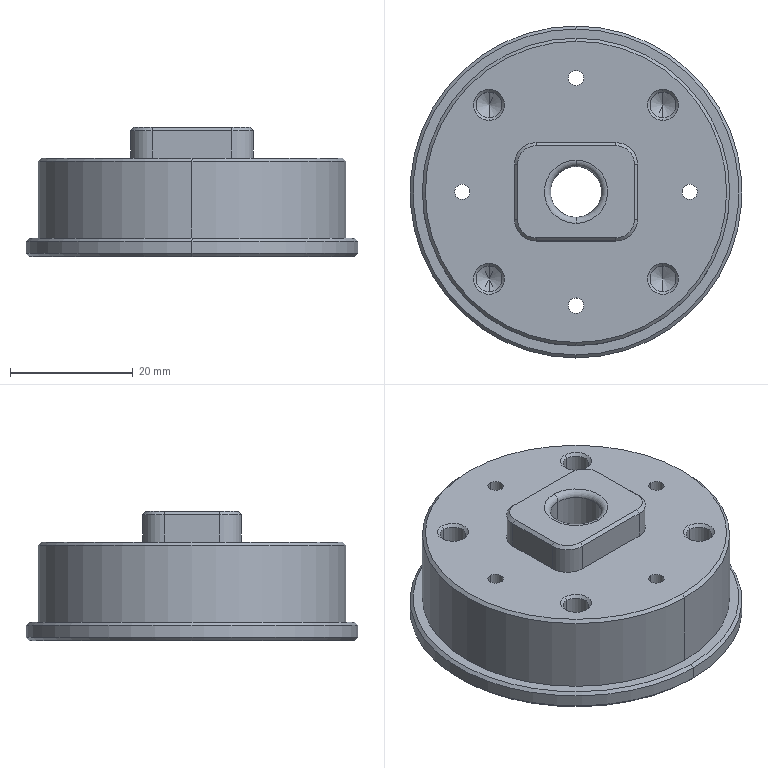NC program | NX | posted with a generic post | part box 54 x 54 x 21 mm
Lines 1 to 245 of 9691:
N10 G17 G21 G94 G90
(FLOOR_WALL_COPY , TOOL : D80)
N12 T19 M6
N14 G54
N16 G17 G0 G90 X75. Y0. S6500 M3
N18 G43 Z30. H19
N20 Z7.
N22 G94 G1 Z4. F1500.
N24 X72.
N26 X-72.
N28 X-75.
N30 Z7.
N32 G0 Z30.
N34 X75.
N36 Z6.
N38 G1 Z3.
N40 X72.
N42 X-72.
N44 X-75.
N46 Z6.
N48 G0 Z30.
N50 X75.
N52 Z5.
N54 G1 Z2.
N56 X72.
N58 X-72.
N60 X-75.
N62 Z5.
N64 G0 Z30.
N66 X75.
N68 Z4.
N70 G1 Z1.
N72 X72.
N74 X-72.
N76 X-75.
N78 Z4.
N80 G0 Z30.
N82 X75.
N84 Z3.
N86 G1 Z0.
N88 X72.
N90 X-72.
N92 X-75.
N94 Z3.
N96 G0 Z30.
N98 M5
(HOLE_MILLING_COPY , TOOL : D6)
N100 T12 M6
N102 G54
N104 G17 G0 G90 X0. Y0. S9500 M3
N106 G43 Z30. H12
N108 Z0.5
N110 G94 G3 X-0.725 Y0.725 R0.725 F1200.
N112 X-1.45 Y0. R0.725
N114 X-1.45 Y0. Z0. I1.45 J0.
N116 X-1.45 Y0. Z-0.5 I1.45 J0.
N118 X-1.45 Y0. Z-1. I1.45 J0.
N120 X-1.45 Y0. Z-1.5 I1.45 J0.
N122 X-1.45 Y0. Z-2. I1.45 J0.
N124 X-1.45 Y0. Z-2.5 I1.45 J0.
N126 X0. Y-1.45 R1.45
N128 X-1.45 Y0. R-1.45
N130 X-0.725 Y-0.725 R0.725
N132 X0. Y0. R0.725
N134 G0 Z30.
(FLOOR_WALL_1 , TOOL : D6)
N136 X-0.147 Y-2.
N138 Z1.5
N140 G1 X0.348 Z1.474 F1250.
N142 X1.114 Y-1.697 Z1.431
N144 X1.697 Y-1.114 Z1.388
N146 X2. Y-0.348 Z1.345
N148 Y0.348 Z1.308
N150 X1.697 Y1.114 Z1.265
N152 X1.114 Y1.697 Z1.222
N154 X0.348 Y2. Z1.178
N156 X-0.348 Z1.142
N158 X-1.114 Y1.697 Z1.099
N160 X-1.697 Y1.114 Z1.056
N162 X-2. Y0.348 Z1.012
N164 Y-0.348 Z0.976
N166 X-1.697 Y-1.114 Z0.933
N168 X-1.114 Y-1.697 Z0.89
N170 X-0.348 Y-2. Z0.846
N172 X0.348 Z0.81
N174 X1.114 Y-1.697 Z0.767
N176 X1.697 Y-1.114 Z0.724
N178 X2. Y-0.348 Z0.68
N180 Y0.348 Z0.644
N182 X1.697 Y1.114 Z0.601
N184 X1.114 Y1.697 Z0.558
N186 X0.348 Y2. Z0.514
N188 X-0.348 Z0.478
N190 X-1.114 Y1.697 Z0.435
N192 X-1.697 Y1.114 Z0.392
N194 X-2. Y0.348 Z0.348
N196 Y-0.348 Z0.312
N198 X-1.697 Y-1.114 Z0.269
N200 X-1.114 Y-1.697 Z0.226
N202 X-0.348 Y-2. Z0.182
N204 X0.348 Z0.146
N206 X1.114 Y-1.697 Z0.103
N208 X1.697 Y-1.114 Z0.059
N210 X2. Y-0.348 Z0.016
N212 Y0.348 Z-0.02
N214 X1.697 Y1.114 Z-0.063
N216 X1.114 Y1.697 Z-0.107
N218 X0.348 Y2. Z-0.15
N220 X-0.348 Z-0.186
N222 X-1.114 Y1.697 Z-0.229
N224 X-1.697 Y1.114 Z-0.273
N226 X-2. Y0.348 Z-0.316
N228 Y-0.348 Z-0.352
N230 X-1.697 Y-1.114 Z-0.395
N232 X-1.114 Y-1.697 Z-0.439
N234 X-0.348 Y-2. Z-0.482
N236 X0. Z-0.5
N238 G3 X2. Y0. R2.
N240 X0. Y-2. R-2.
N242 G1 Y-5.
N244 G3 X5. Y0. R5.
N246 X0. Y-5. R-5.
N248 G1 Z1.
N250 G0 X-0.147 Y-2.
N252 G1 X0.348 Z0.974
N254 X1.114 Y-1.697 Z0.931
N256 X1.697 Y-1.114 Z0.888
N258 X2. Y-0.348 Z0.845
N260 Y0.348 Z0.808
N262 X1.697 Y1.114 Z0.765
N264 X1.114 Y1.697 Z0.722
N266 X0.348 Y2. Z0.678
N268 X-0.348 Z0.642
N270 X-1.114 Y1.697 Z0.599
N272 X-1.697 Y1.114 Z0.556
N274 X-2. Y0.348 Z0.512
N276 Y-0.348 Z0.476
N278 X-1.697 Y-1.114 Z0.433
N280 X-1.114 Y-1.697 Z0.39
N282 X-0.348 Y-2. Z0.346
N284 X0.348 Z0.31
N286 X1.114 Y-1.697 Z0.267
N288 X1.697 Y-1.114 Z0.224
N290 X2. Y-0.348 Z0.18
N292 Y0.348 Z0.144
N294 X1.697 Y1.114 Z0.101
N296 X1.114 Y1.697 Z0.058
N298 X0.348 Y2. Z0.014
N300 X-0.348 Z-0.022
N302 X-1.114 Y1.697 Z-0.065
N304 X-1.697 Y1.114 Z-0.108
N306 X-2. Y0.348 Z-0.152
N308 Y-0.348 Z-0.188
N310 X-1.697 Y-1.114 Z-0.231
N312 X-1.114 Y-1.697 Z-0.274
N314 X-0.348 Y-2. Z-0.318
N316 X0.348 Z-0.354
N318 X1.114 Y-1.697 Z-0.397
N320 X1.697 Y-1.114 Z-0.441
N322 X2. Y-0.348 Z-0.484
N324 Y0.348 Z-0.52
N326 X1.697 Y1.114 Z-0.563
N328 X1.114 Y1.697 Z-0.607
N330 X0.348 Y2. Z-0.65
N332 X-0.348 Z-0.686
N334 X-1.114 Y1.697 Z-0.729
N336 X-1.697 Y1.114 Z-0.773
N338 X-2. Y0.348 Z-0.816
N340 Y-0.348 Z-0.852
N342 X-1.697 Y-1.114 Z-0.895
N344 X-1.114 Y-1.697 Z-0.939
N346 X-0.348 Y-2. Z-0.982
N348 X0. Z-1.
N350 G3 X2. Y0. R2.
N352 X0. Y-2. R-2.
N354 G1 Y-5.
N356 G3 X5. Y0. R5.
N358 X0. Y-5. R-5.
N360 G1 Z0.5
N362 G0 X-0.147 Y-2.
N364 G1 X0.348 Z0.474
N366 X1.114 Y-1.697 Z0.431
N368 X1.697 Y-1.114 Z0.388
N370 X2. Y-0.348 Z0.345
N372 Y0.348 Z0.308
N374 X1.697 Y1.114 Z0.265
N376 X1.114 Y1.697 Z0.222
N378 X0.348 Y2. Z0.178
N380 X-0.348 Z0.142
N382 X-1.114 Y1.697 Z0.099
N384 X-1.697 Y1.114 Z0.056
N386 X-2. Y0.348 Z0.012
N388 Y-0.348 Z-0.024
N390 X-1.697 Y-1.114 Z-0.067
N392 X-1.114 Y-1.697 Z-0.11
N394 X-0.348 Y-2. Z-0.154
N396 X0.348 Z-0.19
N398 X1.114 Y-1.697 Z-0.233
N400 X1.697 Y-1.114 Z-0.276
N402 X2. Y-0.348 Z-0.32
N404 Y0.348 Z-0.356
N406 X1.697 Y1.114 Z-0.399
N408 X1.114 Y1.697 Z-0.442
N410 X0.348 Y2. Z-0.486
N412 X-0.348 Z-0.522
N414 X-1.114 Y1.697 Z-0.565
N416 X-1.697 Y1.114 Z-0.608
N418 X-2. Y0.348 Z-0.652
N420 Y-0.348 Z-0.688
N422 X-1.697 Y-1.114 Z-0.731
N424 X-1.114 Y-1.697 Z-0.774
N426 X-0.348 Y-2. Z-0.818
N428 X0.348 Z-0.854
N430 X1.114 Y-1.697 Z-0.897
N432 X1.697 Y-1.114 Z-0.941
N434 X2. Y-0.348 Z-0.984
N436 Y0.348 Z-1.02
N438 X1.697 Y1.114 Z-1.063
N440 X1.114 Y1.697 Z-1.107
N442 X0.348 Y2. Z-1.15
N444 X-0.348 Z-1.186
N446 X-1.114 Y1.697 Z-1.229
N448 X-1.697 Y1.114 Z-1.273
N450 X-2. Y0.348 Z-1.316
N452 Y-0.348 Z-1.352
N454 X-1.697 Y-1.114 Z-1.395
N456 X-1.114 Y-1.697 Z-1.439
N458 X-0.348 Y-2. Z-1.482
N460 X0. Z-1.5
N462 G3 X2. Y0. R2.
N464 X0. Y-2. R-2.
N466 G1 Y-5.
N468 G3 X5. Y0. R5.
N470 X0. Y-5. R-5.
N472 G1 Z0.
N474 G0 Z30.
N476 M5